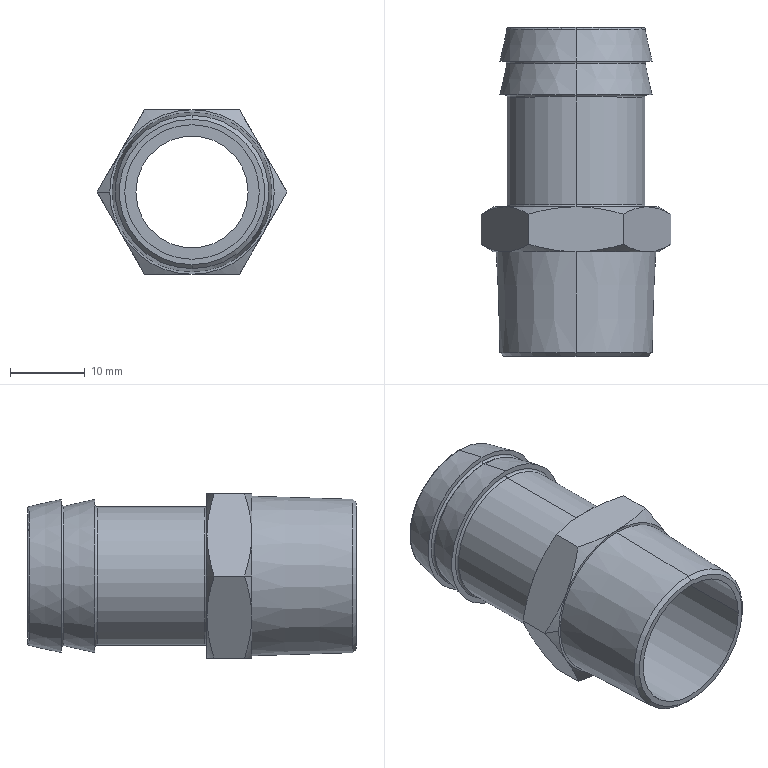Part | SolidWorks | features BaseBody 1 | 1 solid | 54 faces | box 25.403 x 44 x 22 mm | volume 3954 mm3 | cone 22 | plane 14 | torus 10 | cylinder 8 | commonest cylinder face diameters 15 x2 17 x2 18 x2 18.5 x2